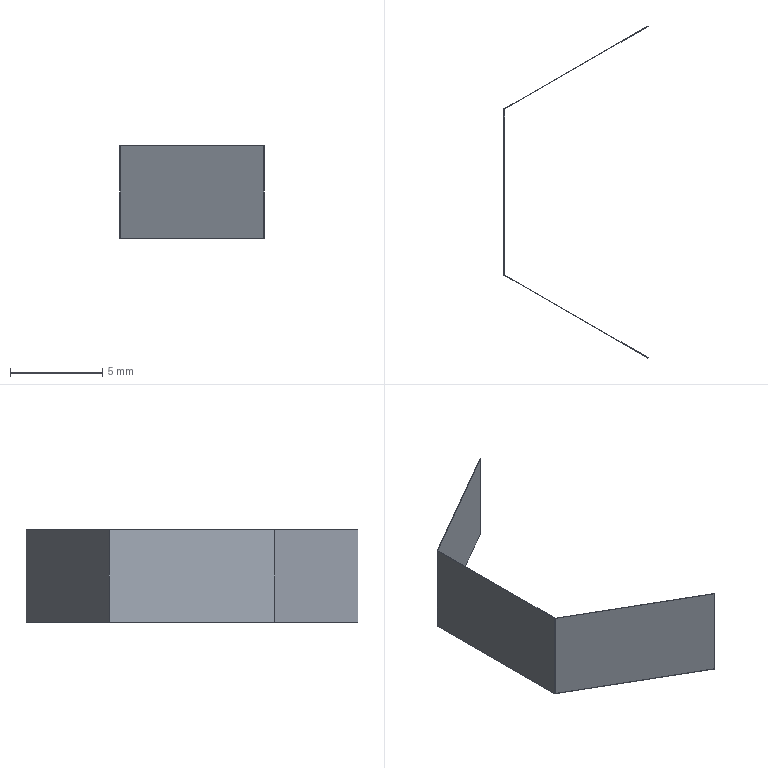Part | STEP file | 1 solid | 10 faces | box 7.817 x 18 x 5 mm | volume 4.038 mm3 | plane 10
STEP:
#1=CARTESIAN_POINT('',(0.,0.,0.));
#2=DIRECTION('',(0.,0.,1.));
#3=DIRECTION('',(1.,0.,0.));
#4=AXIS2_PLACEMENT_3D('',#1,#2,#3);
#5=CARTESIAN_POINT('',(23.783,162.32,44.99));
#6=VERTEX_POINT('',#5);
#7=CARTESIAN_POINT('',(23.783,162.32,39.99));
#8=VERTEX_POINT('',#7);
#9=CARTESIAN_POINT('',(23.783,162.32,44.99));
#10=DIRECTION('',(0.,0.,-1.));
#11=VECTOR('',#10,1.);
#12=LINE('',#9,#11);
#13=CARTESIAN_POINT('',(31.577,166.82,44.99));
#14=DIRECTION('',(0.5,-0.866,0.));
#15=DIRECTION('',(0.866,0.5,0.));
#16=AXIS2_PLACEMENT_3D('',#13,#14,#15);
#17=PLANE('',#16);
#18=CARTESIAN_POINT('',(-9.,0.));
#19=DIRECTION('',(0.,-1.));
#20=VECTOR('',#19,1.);
#21=LINE('',#18,#20);
#22=(GEOMETRIC_REPRESENTATION_CONTEXT(2)PARAMETRIC_REPRESENTATION_CONTEXT()REPRESENTATION_CONTEXT('',''));
#23=DEFINITIONAL_REPRESENTATION('',(#21),#22);
#24=PCURVE('',#17,#23);
#25=CARTESIAN_POINT('',(23.783,162.32,44.99));
#26=DIRECTION('',(1.,0.,0.));
#27=DIRECTION('',(0.,0.,-1.));
#28=AXIS2_PLACEMENT_3D('',#25,#26,#27);
#29=PLANE('',#28);
#30=CARTESIAN_POINT('',(0.,0.));
#31=DIRECTION('',(1.,0.));
#32=VECTOR('',#31,1.);
#33=LINE('',#30,#32);
#34=(GEOMETRIC_REPRESENTATION_CONTEXT(2)PARAMETRIC_REPRESENTATION_CONTEXT()REPRESENTATION_CONTEXT('',''));
#35=DEFINITIONAL_REPRESENTATION('',(#33),#34);
#36=PCURVE('',#29,#35);
#37=SURFACE_CURVE('',#12,(#24,#36),.PCURVE_S1.);
#38=EDGE_CURVE('',#6,#8,#37,.T.);
#39=ORIENTED_EDGE('',*,*,#38,.F.);
#40=CARTESIAN_POINT('',(31.577,166.82,44.99));
#41=VERTEX_POINT('',#40);
#42=CARTESIAN_POINT('',(31.577,166.82,44.99));
#43=DIRECTION('',(-0.866,-0.5,0.));
#44=VECTOR('',#43,1.);
#45=LINE('',#42,#44);
#46=CARTESIAN_POINT('',(0.,0.));
#47=DIRECTION('',(-1.,0.));
#48=VECTOR('',#47,1.);
#49=LINE('',#46,#48);
#50=(GEOMETRIC_REPRESENTATION_CONTEXT(2)PARAMETRIC_REPRESENTATION_CONTEXT()REPRESENTATION_CONTEXT('',''));
#51=DEFINITIONAL_REPRESENTATION('',(#49),#50);
#52=PCURVE('',#17,#51);
#53=CARTESIAN_POINT('',(31.622,157.82,44.99));
#54=DIRECTION('',(0.,0.,-1.));
#55=DIRECTION('',(-1.,0.,0.));
#56=AXIS2_PLACEMENT_3D('',#53,#54,#55);
#57=PLANE('',#56);
#58=CARTESIAN_POINT('',(0.0449,9.));
#59=DIRECTION('',(0.866,-0.5));
#60=VECTOR('',#59,1.);
#61=LINE('',#58,#60);
#62=(GEOMETRIC_REPRESENTATION_CONTEXT(2)PARAMETRIC_REPRESENTATION_CONTEXT()REPRESENTATION_CONTEXT('',''));
#63=DEFINITIONAL_REPRESENTATION('',(#61),#62);
#64=PCURVE('',#57,#63);
#65=SURFACE_CURVE('',#45,(#52,#64),.PCURVE_S1.);
#66=EDGE_CURVE('',#41,#6,#65,.T.);
#67=ORIENTED_EDGE('',*,*,#66,.F.);
#68=CARTESIAN_POINT('',(31.577,166.82,39.99));
#69=VERTEX_POINT('',#68);
#70=CARTESIAN_POINT('',(31.577,166.82,44.99));
#71=DIRECTION('',(0.,0.,1.));
#72=VECTOR('',#71,1.);
#73=LINE('',#70,#72);
#74=CARTESIAN_POINT('',(0.,0.));
#75=DIRECTION('',(0.,1.));
#76=VECTOR('',#75,1.);
#77=LINE('',#74,#76);
#78=(GEOMETRIC_REPRESENTATION_CONTEXT(2)PARAMETRIC_REPRESENTATION_CONTEXT()REPRESENTATION_CONTEXT('',''));
#79=DEFINITIONAL_REPRESENTATION('',(#77),#78);
#80=PCURVE('',#17,#79);
#81=CARTESIAN_POINT('',(39.371,162.32,44.99));
#82=DIRECTION('',(-0.5,-0.866,0.));
#83=DIRECTION('',(0.866,-0.5,0.));
#84=AXIS2_PLACEMENT_3D('',#81,#82,#83);
#85=PLANE('',#84);
#86=CARTESIAN_POINT('',(-9.,0.));
#87=DIRECTION('',(0.,1.));
#88=VECTOR('',#87,1.);
#89=LINE('',#86,#88);
#90=(GEOMETRIC_REPRESENTATION_CONTEXT(2)PARAMETRIC_REPRESENTATION_CONTEXT()REPRESENTATION_CONTEXT('',''));
#91=DEFINITIONAL_REPRESENTATION('',(#89),#90);
#92=PCURVE('',#85,#91);
#93=SURFACE_CURVE('',#73,(#80,#92),.PCURVE_S1.);
#94=EDGE_CURVE('',#69,#41,#93,.T.);
#95=ORIENTED_EDGE('',*,*,#94,.F.);
#96=CARTESIAN_POINT('',(31.577,166.82,39.99));
#97=DIRECTION('',(0.866,0.5,0.));
#98=VECTOR('',#97,1.);
#99=LINE('',#96,#98);
#100=CARTESIAN_POINT('',(0.,-5.));
#101=DIRECTION('',(1.,0.));
#102=VECTOR('',#101,1.);
#103=LINE('',#100,#102);
#104=(GEOMETRIC_REPRESENTATION_CONTEXT(2)PARAMETRIC_REPRESENTATION_CONTEXT()REPRESENTATION_CONTEXT('',''));
#105=DEFINITIONAL_REPRESENTATION('',(#103),#104);
#106=PCURVE('',#17,#105);
#107=CARTESIAN_POINT('',(31.622,166.745,39.99));
#108=DIRECTION('',(0.,0.,1.));
#109=DIRECTION('',(1.,0.,0.));
#110=AXIS2_PLACEMENT_3D('',#107,#108,#109);
#111=PLANE('',#110);
#112=CARTESIAN_POINT('',(-0.0449,0.075));
#113=DIRECTION('',(0.866,0.5));
#114=VECTOR('',#113,1.);
#115=LINE('',#112,#114);
#116=(GEOMETRIC_REPRESENTATION_CONTEXT(2)PARAMETRIC_REPRESENTATION_CONTEXT()REPRESENTATION_CONTEXT('',''));
#117=DEFINITIONAL_REPRESENTATION('',(#115),#116);
#118=PCURVE('',#111,#117);
#119=SURFACE_CURVE('',#99,(#106,#118),.PCURVE_S1.);
#120=EDGE_CURVE('',#8,#69,#119,.T.);
#121=ORIENTED_EDGE('',*,*,#120,.F.);
#122=EDGE_LOOP('',(#39,#67,#95,#121));
#123=FACE_BOUND('',#122,.T.);
#124=ADVANCED_FACE('',(#123),#17,.F.);
#125=CARTESIAN_POINT('',(23.783,153.32,39.99));
#126=VERTEX_POINT('',#125);
#127=CARTESIAN_POINT('',(31.577,148.82,39.99));
#128=VERTEX_POINT('',#127);
#129=CARTESIAN_POINT('',(23.783,153.32,39.99));
#130=DIRECTION('',(0.866,-0.5,0.));
#131=VECTOR('',#130,1.);
#132=LINE('',#129,#131);
#133=CARTESIAN_POINT('',(-7.839,-13.425));
#134=DIRECTION('',(0.866,-0.5));
#135=VECTOR('',#134,1.);
#136=LINE('',#133,#135);
#137=(GEOMETRIC_REPRESENTATION_CONTEXT(2)PARAMETRIC_REPRESENTATION_CONTEXT()REPRESENTATION_CONTEXT('',''));
#138=DEFINITIONAL_REPRESENTATION('',(#136),#137);
#139=PCURVE('',#111,#138);
#140=CARTESIAN_POINT('',(23.783,153.32,44.99));
#141=DIRECTION('',(0.5,0.866,0.));
#142=DIRECTION('',(-0.866,0.5,0.));
#143=AXIS2_PLACEMENT_3D('',#140,#141,#142);
#144=PLANE('',#143);
#145=CARTESIAN_POINT('',(0.,-5.));
#146=DIRECTION('',(-1.,0.));
#147=VECTOR('',#146,1.);
#148=LINE('',#145,#147);
#149=(GEOMETRIC_REPRESENTATION_CONTEXT(2)PARAMETRIC_REPRESENTATION_CONTEXT()REPRESENTATION_CONTEXT('',''));
#150=DEFINITIONAL_REPRESENTATION('',(#148),#149);
#151=PCURVE('',#144,#150);
#152=SURFACE_CURVE('',#132,(#139,#151),.PCURVE_S1.);
#153=EDGE_CURVE('',#126,#128,#152,.T.);
#154=ORIENTED_EDGE('',*,*,#153,.F.);
#155=CARTESIAN_POINT('',(23.783,166.745,39.99));
#156=DIRECTION('',(0.,-1.,0.));
#157=VECTOR('',#156,1.);
#158=LINE('',#155,#157);
#159=CARTESIAN_POINT('',(-7.839,0.));
#160=DIRECTION('',(0.,-1.));
#161=VECTOR('',#160,1.);
#162=LINE('',#159,#161);
#163=(GEOMETRIC_REPRESENTATION_CONTEXT(2)PARAMETRIC_REPRESENTATION_CONTEXT()REPRESENTATION_CONTEXT('',''));
#164=DEFINITIONAL_REPRESENTATION('',(#162),#163);
#165=PCURVE('',#111,#164);
#166=CARTESIAN_POINT('',(5.,4.425));
#167=DIRECTION('',(0.,-1.));
#168=VECTOR('',#167,1.);
#169=LINE('',#166,#168);
#170=(GEOMETRIC_REPRESENTATION_CONTEXT(2)PARAMETRIC_REPRESENTATION_CONTEXT()REPRESENTATION_CONTEXT('',''));
#171=DEFINITIONAL_REPRESENTATION('',(#169),#170);
#172=PCURVE('',#29,#171);
#173=SURFACE_CURVE('',#158,(#165,#172),.PCURVE_S1.);
#174=EDGE_CURVE('',#8,#126,#173,.T.);
#175=ORIENTED_EDGE('',*,*,#174,.F.);
#176=ORIENTED_EDGE('',*,*,#120,.T.);
#177=CARTESIAN_POINT('',(31.6,166.807,39.99));
#178=VERTEX_POINT('',#177);
#179=CARTESIAN_POINT('',(31.6,166.807,39.99));
#180=DIRECTION('',(-0.866,0.5,0.));
#181=VECTOR('',#180,1.);
#182=LINE('',#179,#181);
#183=CARTESIAN_POINT('',(-0.02245,0.06204));
#184=DIRECTION('',(-0.866,0.5));
#185=VECTOR('',#184,1.);
#186=LINE('',#183,#185);
#187=(GEOMETRIC_REPRESENTATION_CONTEXT(2)PARAMETRIC_REPRESENTATION_CONTEXT()REPRESENTATION_CONTEXT('',''));
#188=DEFINITIONAL_REPRESENTATION('',(#186),#187);
#189=PCURVE('',#111,#188);
#190=CARTESIAN_POINT('',(-8.974,-5.));
#191=DIRECTION('',(-1.,0.));
#192=VECTOR('',#191,1.);
#193=LINE('',#190,#192);
#194=(GEOMETRIC_REPRESENTATION_CONTEXT(2)PARAMETRIC_REPRESENTATION_CONTEXT()REPRESENTATION_CONTEXT('',''));
#195=DEFINITIONAL_REPRESENTATION('',(#193),#194);
#196=PCURVE('',#85,#195);
#197=SURFACE_CURVE('',#182,(#189,#196),.PCURVE_S1.);
#198=EDGE_CURVE('',#178,#69,#197,.T.);
#199=ORIENTED_EDGE('',*,*,#198,.F.);
#200=CARTESIAN_POINT('',(23.828,162.32,39.99));
#201=VERTEX_POINT('',#200);
#202=CARTESIAN_POINT('',(23.828,162.32,39.99));
#203=DIRECTION('',(0.866,0.5,0.));
#204=VECTOR('',#203,1.);
#205=LINE('',#202,#204);
#206=CARTESIAN_POINT('',(-7.794,-4.425));
#207=DIRECTION('',(0.866,0.5));
#208=VECTOR('',#207,1.);
#209=LINE('',#206,#208);
#210=(GEOMETRIC_REPRESENTATION_CONTEXT(2)PARAMETRIC_REPRESENTATION_CONTEXT()REPRESENTATION_CONTEXT('',''));
#211=DEFINITIONAL_REPRESENTATION('',(#209),#210);
#212=PCURVE('',#111,#211);
#213=CARTESIAN_POINT('',(23.828,162.32,39.99));
#214=DIRECTION('',(-0.5,0.866,0.));
#215=DIRECTION('',(-0.866,-0.5,0.));
#216=AXIS2_PLACEMENT_3D('',#213,#214,#215);
#217=PLANE('',#216);
#218=CARTESIAN_POINT('',(0.,0.));
#219=DIRECTION('',(-1.,0.));
#220=VECTOR('',#219,1.);
#221=LINE('',#218,#220);
#222=(GEOMETRIC_REPRESENTATION_CONTEXT(2)PARAMETRIC_REPRESENTATION_CONTEXT()REPRESENTATION_CONTEXT('',''));
#223=DEFINITIONAL_REPRESENTATION('',(#221),#222);
#224=PCURVE('',#217,#223);
#225=SURFACE_CURVE('',#205,(#212,#224),.PCURVE_S1.);
#226=EDGE_CURVE('',#201,#178,#225,.T.);
#227=ORIENTED_EDGE('',*,*,#226,.F.);
#228=CARTESIAN_POINT('',(23.828,153.32,39.99));
#229=VERTEX_POINT('',#228);
#230=CARTESIAN_POINT('',(23.828,166.745,39.99));
#231=DIRECTION('',(0.,1.,0.));
#232=VECTOR('',#231,1.);
#233=LINE('',#230,#232);
#234=CARTESIAN_POINT('',(-7.794,0.));
#235=DIRECTION('',(0.,1.));
#236=VECTOR('',#235,1.);
#237=LINE('',#234,#236);
#238=(GEOMETRIC_REPRESENTATION_CONTEXT(2)PARAMETRIC_REPRESENTATION_CONTEXT()REPRESENTATION_CONTEXT('',''));
#239=DEFINITIONAL_REPRESENTATION('',(#237),#238);
#240=PCURVE('',#111,#239);
#241=CARTESIAN_POINT('',(23.828,153.32,39.99));
#242=DIRECTION('',(-1.,0.,0.));
#243=DIRECTION('',(0.,0.,1.));
#244=AXIS2_PLACEMENT_3D('',#241,#242,#243);
#245=PLANE('',#244);
#246=CARTESIAN_POINT('',(0.,13.425));
#247=DIRECTION('',(0.,1.));
#248=VECTOR('',#247,1.);
#249=LINE('',#246,#248);
#250=(GEOMETRIC_REPRESENTATION_CONTEXT(2)PARAMETRIC_REPRESENTATION_CONTEXT()REPRESENTATION_CONTEXT('',''));
#251=DEFINITIONAL_REPRESENTATION('',(#249),#250);
#252=PCURVE('',#245,#251);
#253=SURFACE_CURVE('',#233,(#240,#252),.PCURVE_S1.);
#254=EDGE_CURVE('',#229,#201,#253,.T.);
#255=ORIENTED_EDGE('',*,*,#254,.F.);
#256=CARTESIAN_POINT('',(31.6,148.833,39.99));
#257=VERTEX_POINT('',#256);
#258=CARTESIAN_POINT('',(31.6,148.833,39.99));
#259=DIRECTION('',(-0.866,0.5,0.));
#260=VECTOR('',#259,1.);
#261=LINE('',#258,#260);
#262=CARTESIAN_POINT('',(-0.02245,-17.912));
#263=DIRECTION('',(-0.866,0.5));
#264=VECTOR('',#263,1.);
#265=LINE('',#262,#264);
#266=(GEOMETRIC_REPRESENTATION_CONTEXT(2)PARAMETRIC_REPRESENTATION_CONTEXT()REPRESENTATION_CONTEXT('',''));
#267=DEFINITIONAL_REPRESENTATION('',(#265),#266);
#268=PCURVE('',#111,#267);
#269=CARTESIAN_POINT('',(31.622,148.82,39.99));
#270=DIRECTION('',(-0.5,-0.866,0.));
#271=DIRECTION('',(0.866,-0.5,0.));
#272=AXIS2_PLACEMENT_3D('',#269,#270,#271);
#273=PLANE('',#272);
#274=CARTESIAN_POINT('',(-0.02592,0.));
#275=DIRECTION('',(-1.,0.));
#276=VECTOR('',#275,1.);
#277=LINE('',#274,#276);
#278=(GEOMETRIC_REPRESENTATION_CONTEXT(2)PARAMETRIC_REPRESENTATION_CONTEXT()REPRESENTATION_CONTEXT('',''));
#279=DEFINITIONAL_REPRESENTATION('',(#277),#278);
#280=PCURVE('',#273,#279);
#281=SURFACE_CURVE('',#261,(#268,#280),.PCURVE_S1.);
#282=EDGE_CURVE('',#257,#229,#281,.T.);
#283=ORIENTED_EDGE('',*,*,#282,.F.);
#284=CARTESIAN_POINT('',(31.577,148.82,39.99));
#285=DIRECTION('',(-0.866,-0.5,0.));
#286=VECTOR('',#285,1.);
#287=LINE('',#284,#286);
#288=CARTESIAN_POINT('',(-0.0449,-17.925));
#289=DIRECTION('',(-0.866,-0.5));
#290=VECTOR('',#289,1.);
#291=LINE('',#288,#290);
#292=(GEOMETRIC_REPRESENTATION_CONTEXT(2)PARAMETRIC_REPRESENTATION_CONTEXT()REPRESENTATION_CONTEXT('',''));
#293=DEFINITIONAL_REPRESENTATION('',(#291),#292);
#294=PCURVE('',#111,#293);
#295=CARTESIAN_POINT('',(31.577,148.82,44.99));
#296=DIRECTION('',(-0.5,0.866,0.));
#297=DIRECTION('',(-0.866,-0.5,0.));
#298=AXIS2_PLACEMENT_3D('',#295,#296,#297);
#299=PLANE('',#298);
#300=CARTESIAN_POINT('',(0.,-5.));
#301=DIRECTION('',(1.,0.));
#302=VECTOR('',#301,1.);
#303=LINE('',#300,#302);
#304=(GEOMETRIC_REPRESENTATION_CONTEXT(2)PARAMETRIC_REPRESENTATION_CONTEXT()REPRESENTATION_CONTEXT('',''));
#305=DEFINITIONAL_REPRESENTATION('',(#303),#304);
#306=PCURVE('',#299,#305);
#307=SURFACE_CURVE('',#287,(#294,#306),.PCURVE_S1.);
#308=EDGE_CURVE('',#257,#128,#307,.T.);
#309=ORIENTED_EDGE('',*,*,#308,.T.);
#310=EDGE_LOOP('',(#154,#175,#176,#199,#227,#255,#283,#309));
#311=FACE_BOUND('',#310,.T.);
#312=ADVANCED_FACE('',(#311),#111,.F.);
#313=CARTESIAN_POINT('',(23.783,153.32,44.99));
#314=VERTEX_POINT('',#313);
#315=CARTESIAN_POINT('',(23.783,153.32,44.99));
#316=DIRECTION('',(0.,0.,-1.));
#317=VECTOR('',#316,1.);
#318=LINE('',#315,#317);
#319=CARTESIAN_POINT('',(0.,-9.));
#320=DIRECTION('',(1.,0.));
#321=VECTOR('',#320,1.);
#322=LINE('',#319,#321);
#323=(GEOMETRIC_REPRESENTATION_CONTEXT(2)PARAMETRIC_REPRESENTATION_CONTEXT()REPRESENTATION_CONTEXT('',''));
#324=DEFINITIONAL_REPRESENTATION('',(#322),#323);
#325=PCURVE('',#29,#324);
#326=CARTESIAN_POINT('',(0.,0.));
#327=DIRECTION('',(0.,-1.));
#328=VECTOR('',#327,1.);
#329=LINE('',#326,#328);
#330=(GEOMETRIC_REPRESENTATION_CONTEXT(2)PARAMETRIC_REPRESENTATION_CONTEXT()REPRESENTATION_CONTEXT('',''));
#331=DEFINITIONAL_REPRESENTATION('',(#329),#330);
#332=PCURVE('',#144,#331);
#333=SURFACE_CURVE('',#318,(#325,#332),.PCURVE_S1.);
#334=EDGE_CURVE('',#314,#126,#333,.T.);
#335=ORIENTED_EDGE('',*,*,#334,.F.);
#336=CARTESIAN_POINT('',(23.783,162.32,44.99));
#337=DIRECTION('',(0.,-1.,0.));
#338=VECTOR('',#337,1.);
#339=LINE('',#336,#338);
#340=CARTESIAN_POINT('',(0.,0.));
#341=DIRECTION('',(0.,-1.));
#342=VECTOR('',#341,1.);
#343=LINE('',#340,#342);
#344=(GEOMETRIC_REPRESENTATION_CONTEXT(2)PARAMETRIC_REPRESENTATION_CONTEXT()REPRESENTATION_CONTEXT('',''));
#345=DEFINITIONAL_REPRESENTATION('',(#343),#344);
#346=PCURVE('',#29,#345);
#347=CARTESIAN_POINT('',(7.839,4.5));
#348=DIRECTION('',(0.,-1.));
#349=VECTOR('',#348,1.);
#350=LINE('',#347,#349);
#351=(GEOMETRIC_REPRESENTATION_CONTEXT(2)PARAMETRIC_REPRESENTATION_CONTEXT()REPRESENTATION_CONTEXT('',''));
#352=DEFINITIONAL_REPRESENTATION('',(#350),#351);
#353=PCURVE('',#57,#352);
#354=SURFACE_CURVE('',#339,(#346,#353),.PCURVE_S1.);
#355=EDGE_CURVE('',#6,#314,#354,.T.);
#356=ORIENTED_EDGE('',*,*,#355,.F.);
#357=ORIENTED_EDGE('',*,*,#38,.T.);
#358=ORIENTED_EDGE('',*,*,#174,.T.);
#359=EDGE_LOOP('',(#335,#356,#357,#358));
#360=FACE_BOUND('',#359,.T.);
#361=ADVANCED_FACE('',(#360),#29,.F.);
#362=CARTESIAN_POINT('',(23.828,153.32,44.99));
#363=VERTEX_POINT('',#362);
#364=CARTESIAN_POINT('',(31.6,148.833,44.99));
#365=VERTEX_POINT('',#364);
#366=CARTESIAN_POINT('',(23.828,153.32,44.99));
#367=DIRECTION('',(0.866,-0.5,0.));
#368=VECTOR('',#367,1.);
#369=LINE('',#366,#368);
#370=CARTESIAN_POINT('',(7.794,-4.5));
#371=DIRECTION('',(-0.866,-0.5));
#372=VECTOR('',#371,1.);
#373=LINE('',#370,#372);
#374=(GEOMETRIC_REPRESENTATION_CONTEXT(2)PARAMETRIC_REPRESENTATION_CONTEXT()REPRESENTATION_CONTEXT('',''));
#375=DEFINITIONAL_REPRESENTATION('',(#373),#374);
#376=PCURVE('',#57,#375);
#377=CARTESIAN_POINT('',(-9.,5.));
#378=DIRECTION('',(1.,0.));
#379=VECTOR('',#378,1.);
#380=LINE('',#377,#379);
#381=(GEOMETRIC_REPRESENTATION_CONTEXT(2)PARAMETRIC_REPRESENTATION_CONTEXT()REPRESENTATION_CONTEXT('',''));
#382=DEFINITIONAL_REPRESENTATION('',(#380),#381);
#383=PCURVE('',#273,#382);
#384=SURFACE_CURVE('',#369,(#376,#383),.PCURVE_S1.);
#385=EDGE_CURVE('',#363,#365,#384,.T.);
#386=ORIENTED_EDGE('',*,*,#385,.F.);
#387=CARTESIAN_POINT('',(23.828,162.32,44.99));
#388=VERTEX_POINT('',#387);
#389=CARTESIAN_POINT('',(23.828,157.82,44.99));
#390=DIRECTION('',(0.,-1.,0.));
#391=VECTOR('',#390,1.);
#392=LINE('',#389,#391);
#393=CARTESIAN_POINT('',(7.794,0.));
#394=DIRECTION('',(0.,-1.));
#395=VECTOR('',#394,1.);
#396=LINE('',#393,#395);
#397=(GEOMETRIC_REPRESENTATION_CONTEXT(2)PARAMETRIC_REPRESENTATION_CONTEXT()REPRESENTATION_CONTEXT('',''));
#398=DEFINITIONAL_REPRESENTATION('',(#396),#397);
#399=PCURVE('',#57,#398);
#400=CARTESIAN_POINT('',(5.,4.5));
#401=DIRECTION('',(0.,-1.));
#402=VECTOR('',#401,1.);
#403=LINE('',#400,#402);
#404=(GEOMETRIC_REPRESENTATION_CONTEXT(2)PARAMETRIC_REPRESENTATION_CONTEXT()REPRESENTATION_CONTEXT('',''));
#405=DEFINITIONAL_REPRESENTATION('',(#403),#404);
#406=PCURVE('',#245,#405);
#407=SURFACE_CURVE('',#392,(#399,#406),.PCURVE_S1.);
#408=EDGE_CURVE('',#388,#363,#407,.T.);
#409=ORIENTED_EDGE('',*,*,#408,.F.);
#410=CARTESIAN_POINT('',(31.6,166.807,44.99));
#411=VERTEX_POINT('',#410);
#412=CARTESIAN_POINT('',(31.6,166.807,44.99));
#413=DIRECTION('',(-0.866,-0.5,0.));
#414=VECTOR('',#413,1.);
#415=LINE('',#412,#414);
#416=CARTESIAN_POINT('',(0.02245,8.987));
#417=DIRECTION('',(0.866,-0.5));
#418=VECTOR('',#417,1.);
#419=LINE('',#416,#418);
#420=(GEOMETRIC_REPRESENTATION_CONTEXT(2)PARAMETRIC_REPRESENTATION_CONTEXT()REPRESENTATION_CONTEXT('',''));
#421=DEFINITIONAL_REPRESENTATION('',(#419),#420);
#422=PCURVE('',#57,#421);
#423=CARTESIAN_POINT('',(-8.974,5.));
#424=DIRECTION('',(1.,0.));
#425=VECTOR('',#424,1.);
#426=LINE('',#423,#425);
#427=(GEOMETRIC_REPRESENTATION_CONTEXT(2)PARAMETRIC_REPRESENTATION_CONTEXT()REPRESENTATION_CONTEXT('',''));
#428=DEFINITIONAL_REPRESENTATION('',(#426),#427);
#429=PCURVE('',#217,#428);
#430=SURFACE_CURVE('',#415,(#422,#429),.PCURVE_S1.);
#431=EDGE_CURVE('',#411,#388,#430,.T.);
#432=ORIENTED_EDGE('',*,*,#431,.F.);
#433=CARTESIAN_POINT('',(31.577,166.82,44.99));
#434=DIRECTION('',(0.866,-0.5,0.));
#435=VECTOR('',#434,1.);
#436=LINE('',#433,#435);
#437=CARTESIAN_POINT('',(0.0449,9.));
#438=DIRECTION('',(-0.866,-0.5));
#439=VECTOR('',#438,1.);
#440=LINE('',#437,#439);
#441=(GEOMETRIC_REPRESENTATION_CONTEXT(2)PARAMETRIC_REPRESENTATION_CONTEXT()REPRESENTATION_CONTEXT('',''));
#442=DEFINITIONAL_REPRESENTATION('',(#440),#441);
#443=PCURVE('',#57,#442);
#444=CARTESIAN_POINT('',(-9.,0.));
#445=DIRECTION('',(1.,0.));
#446=VECTOR('',#445,1.);
#447=LINE('',#444,#446);
#448=(GEOMETRIC_REPRESENTATION_CONTEXT(2)PARAMETRIC_REPRESENTATION_CONTEXT()REPRESENTATION_CONTEXT('',''));
#449=DEFINITIONAL_REPRESENTATION('',(#447),#448);
#450=PCURVE('',#85,#449);
#451=SURFACE_CURVE('',#436,(#443,#450),.PCURVE_S1.);
#452=EDGE_CURVE('',#41,#411,#451,.T.);
#453=ORIENTED_EDGE('',*,*,#452,.F.);
#454=ORIENTED_EDGE('',*,*,#66,.T.);
#455=ORIENTED_EDGE('',*,*,#355,.T.);
#456=CARTESIAN_POINT('',(31.577,148.82,44.99));
#457=VERTEX_POINT('',#456);
#458=CARTESIAN_POINT('',(31.577,148.82,44.99));
#459=DIRECTION('',(-0.866,0.5,0.));
#460=VECTOR('',#459,1.);
#461=LINE('',#458,#460);
#462=CARTESIAN_POINT('',(0.0449,-9.));
#463=DIRECTION('',(0.866,0.5));
#464=VECTOR('',#463,1.);
#465=LINE('',#462,#464);
#466=(GEOMETRIC_REPRESENTATION_CONTEXT(2)PARAMETRIC_REPRESENTATION_CONTEXT()REPRESENTATION_CONTEXT('',''));
#467=DEFINITIONAL_REPRESENTATION('',(#465),#466);
#468=PCURVE('',#57,#467);
#469=CARTESIAN_POINT('',(-9.,0.));
#470=DIRECTION('',(1.,0.));
#471=VECTOR('',#470,1.);
#472=LINE('',#469,#471);
#473=(GEOMETRIC_REPRESENTATION_CONTEXT(2)PARAMETRIC_REPRESENTATION_CONTEXT()REPRESENTATION_CONTEXT('',''));
#474=DEFINITIONAL_REPRESENTATION('',(#472),#473);
#475=PCURVE('',#144,#474);
#476=SURFACE_CURVE('',#461,(#468,#475),.PCURVE_S1.);
#477=EDGE_CURVE('',#457,#314,#476,.T.);
#478=ORIENTED_EDGE('',*,*,#477,.F.);
#479=CARTESIAN_POINT('',(31.577,148.82,44.99));
#480=DIRECTION('',(0.866,0.5,0.));
#481=VECTOR('',#480,1.);
#482=LINE('',#479,#481);
#483=CARTESIAN_POINT('',(0.0449,-9.));
#484=DIRECTION('',(-0.866,0.5));
#485=VECTOR('',#484,1.);
#486=LINE('',#483,#485);
#487=(GEOMETRIC_REPRESENTATION_CONTEXT(2)PARAMETRIC_REPRESENTATION_CONTEXT()REPRESENTATION_CONTEXT('',''));
#488=DEFINITIONAL_REPRESENTATION('',(#486),#487);
#489=PCURVE('',#57,#488);
#490=CARTESIAN_POINT('',(0.,0.));
#491=DIRECTION('',(-1.,0.));
#492=VECTOR('',#491,1.);
#493=LINE('',#490,#492);
#494=(GEOMETRIC_REPRESENTATION_CONTEXT(2)PARAMETRIC_REPRESENTATION_CONTEXT()REPRESENTATION_CONTEXT('',''));
#495=DEFINITIONAL_REPRESENTATION('',(#493),#494);
#496=PCURVE('',#299,#495);
#497=SURFACE_CURVE('',#482,(#489,#496),.PCURVE_S1.);
#498=EDGE_CURVE('',#457,#365,#497,.T.);
#499=ORIENTED_EDGE('',*,*,#498,.T.);
#500=EDGE_LOOP('',(#386,#409,#432,#453,#454,#455,#478,#499));
#501=FACE_BOUND('',#500,.T.);
#502=ADVANCED_FACE('',(#501),#57,.F.);
#503=ORIENTED_EDGE('',*,*,#198,.T.);
#504=ORIENTED_EDGE('',*,*,#94,.T.);
#505=ORIENTED_EDGE('',*,*,#452,.T.);
#506=CARTESIAN_POINT('',(31.6,166.807,44.99));
#507=DIRECTION('',(0.,0.,1.));
#508=VECTOR('',#507,1.);
#509=LINE('',#506,#508);
#510=CARTESIAN_POINT('',(-8.974,0.));
#511=DIRECTION('',(0.,1.));
#512=VECTOR('',#511,1.);
#513=LINE('',#510,#512);
#514=(GEOMETRIC_REPRESENTATION_CONTEXT(2)PARAMETRIC_REPRESENTATION_CONTEXT()REPRESENTATION_CONTEXT('',''));
#515=DEFINITIONAL_REPRESENTATION('',(#513),#514);
#516=PCURVE('',#85,#515);
#517=CARTESIAN_POINT('',(-8.974,5.));
#518=DIRECTION('',(0.,1.));
#519=VECTOR('',#518,1.);
#520=LINE('',#517,#519);
#521=(GEOMETRIC_REPRESENTATION_CONTEXT(2)PARAMETRIC_REPRESENTATION_CONTEXT()REPRESENTATION_CONTEXT('',''));
#522=DEFINITIONAL_REPRESENTATION('',(#520),#521);
#523=PCURVE('',#217,#522);
#524=SURFACE_CURVE('',#509,(#516,#523),.PCURVE_S1.);
#525=EDGE_CURVE('',#178,#411,#524,.T.);
#526=ORIENTED_EDGE('',*,*,#525,.F.);
#527=EDGE_LOOP('',(#503,#504,#505,#526));
#528=FACE_BOUND('',#527,.T.);
#529=ADVANCED_FACE('',(#528),#85,.F.);
#530=CARTESIAN_POINT('',(31.577,148.82,44.99));
#531=DIRECTION('',(0.,0.,-1.));
#532=VECTOR('',#531,1.);
#533=LINE('',#530,#532);
#534=CARTESIAN_POINT('',(-9.,0.));
#535=DIRECTION('',(0.,-1.));
#536=VECTOR('',#535,1.);
#537=LINE('',#534,#536);
#538=(GEOMETRIC_REPRESENTATION_CONTEXT(2)PARAMETRIC_REPRESENTATION_CONTEXT()REPRESENTATION_CONTEXT('',''));
#539=DEFINITIONAL_REPRESENTATION('',(#537),#538);
#540=PCURVE('',#144,#539);
#541=CARTESIAN_POINT('',(0.,0.));
#542=DIRECTION('',(0.,-1.));
#543=VECTOR('',#542,1.);
#544=LINE('',#541,#543);
#545=(GEOMETRIC_REPRESENTATION_CONTEXT(2)PARAMETRIC_REPRESENTATION_CONTEXT()REPRESENTATION_CONTEXT('',''));
#546=DEFINITIONAL_REPRESENTATION('',(#544),#545);
#547=PCURVE('',#299,#546);
#548=SURFACE_CURVE('',#533,(#540,#547),.PCURVE_S1.);
#549=EDGE_CURVE('',#457,#128,#548,.T.);
#550=ORIENTED_EDGE('',*,*,#549,.F.);
#551=ORIENTED_EDGE('',*,*,#477,.T.);
#552=ORIENTED_EDGE('',*,*,#334,.T.);
#553=ORIENTED_EDGE('',*,*,#153,.T.);
#554=EDGE_LOOP('',(#550,#551,#552,#553));
#555=FACE_BOUND('',#554,.T.);
#556=ADVANCED_FACE('',(#555),#144,.F.);
#557=ORIENTED_EDGE('',*,*,#431,.T.);
#558=CARTESIAN_POINT('',(23.828,162.32,39.99));
#559=DIRECTION('',(0.,0.,1.));
#560=VECTOR('',#559,1.);
#561=LINE('',#558,#560);
#562=CARTESIAN_POINT('',(0.,0.));
#563=DIRECTION('',(0.,1.));
#564=VECTOR('',#563,1.);
#565=LINE('',#562,#564);
#566=(GEOMETRIC_REPRESENTATION_CONTEXT(2)PARAMETRIC_REPRESENTATION_CONTEXT()REPRESENTATION_CONTEXT('',''));
#567=DEFINITIONAL_REPRESENTATION('',(#565),#566);
#568=PCURVE('',#217,#567);
#569=CARTESIAN_POINT('',(0.,9.));
#570=DIRECTION('',(1.,0.));
#571=VECTOR('',#570,1.);
#572=LINE('',#569,#571);
#573=(GEOMETRIC_REPRESENTATION_CONTEXT(2)PARAMETRIC_REPRESENTATION_CONTEXT()REPRESENTATION_CONTEXT('',''));
#574=DEFINITIONAL_REPRESENTATION('',(#572),#573);
#575=PCURVE('',#245,#574);
#576=SURFACE_CURVE('',#561,(#568,#575),.PCURVE_S1.);
#577=EDGE_CURVE('',#201,#388,#576,.T.);
#578=ORIENTED_EDGE('',*,*,#577,.F.);
#579=ORIENTED_EDGE('',*,*,#226,.T.);
#580=ORIENTED_EDGE('',*,*,#525,.T.);
#581=EDGE_LOOP('',(#557,#578,#579,#580));
#582=FACE_BOUND('',#581,.T.);
#583=ADVANCED_FACE('',(#582),#217,.F.);
#584=CARTESIAN_POINT('',(23.828,153.32,39.99));
#585=DIRECTION('',(0.,0.,1.));
#586=VECTOR('',#585,1.);
#587=LINE('',#584,#586);
#588=CARTESIAN_POINT('',(0.,0.));
#589=DIRECTION('',(1.,0.));
#590=VECTOR('',#589,1.);
#591=LINE('',#588,#590);
#592=(GEOMETRIC_REPRESENTATION_CONTEXT(2)PARAMETRIC_REPRESENTATION_CONTEXT()REPRESENTATION_CONTEXT('',''));
#593=DEFINITIONAL_REPRESENTATION('',(#591),#592);
#594=PCURVE('',#245,#593);
#595=CARTESIAN_POINT('',(-9.,0.));
#596=DIRECTION('',(0.,1.));
#597=VECTOR('',#596,1.);
#598=LINE('',#595,#597);
#599=(GEOMETRIC_REPRESENTATION_CONTEXT(2)PARAMETRIC_REPRESENTATION_CONTEXT()REPRESENTATION_CONTEXT('',''));
#600=DEFINITIONAL_REPRESENTATION('',(#598),#599);
#601=PCURVE('',#273,#600);
#602=SURFACE_CURVE('',#587,(#594,#601),.PCURVE_S1.);
#603=EDGE_CURVE('',#229,#363,#602,.T.);
#604=ORIENTED_EDGE('',*,*,#603,.F.);
#605=ORIENTED_EDGE('',*,*,#254,.T.);
#606=ORIENTED_EDGE('',*,*,#577,.T.);
#607=ORIENTED_EDGE('',*,*,#408,.T.);
#608=EDGE_LOOP('',(#604,#605,#606,#607));
#609=FACE_BOUND('',#608,.T.);
#610=ADVANCED_FACE('',(#609),#245,.F.);
#611=ORIENTED_EDGE('',*,*,#282,.T.);
#612=ORIENTED_EDGE('',*,*,#603,.T.);
#613=ORIENTED_EDGE('',*,*,#385,.T.);
#614=CARTESIAN_POINT('',(31.6,148.833,39.99));
#615=DIRECTION('',(0.,0.,1.));
#616=VECTOR('',#615,1.);
#617=LINE('',#614,#616);
#618=CARTESIAN_POINT('',(-0.02592,0.));
#619=DIRECTION('',(0.,1.));
#620=VECTOR('',#619,1.);
#621=LINE('',#618,#620);
#622=(GEOMETRIC_REPRESENTATION_CONTEXT(2)PARAMETRIC_REPRESENTATION_CONTEXT()REPRESENTATION_CONTEXT('',''));
#623=DEFINITIONAL_REPRESENTATION('',(#621),#622);
#624=PCURVE('',#273,#623);
#625=CARTESIAN_POINT('',(-0.02592,-5.));
#626=DIRECTION('',(0.,1.));
#627=VECTOR('',#626,1.);
#628=LINE('',#625,#627);
#629=(GEOMETRIC_REPRESENTATION_CONTEXT(2)PARAMETRIC_REPRESENTATION_CONTEXT()REPRESENTATION_CONTEXT('',''));
#630=DEFINITIONAL_REPRESENTATION('',(#628),#629);
#631=PCURVE('',#299,#630);
#632=SURFACE_CURVE('',#617,(#624,#631),.PCURVE_S1.);
#633=EDGE_CURVE('',#257,#365,#632,.T.);
#634=ORIENTED_EDGE('',*,*,#633,.F.);
#635=EDGE_LOOP('',(#611,#612,#613,#634));
#636=FACE_BOUND('',#635,.T.);
#637=ADVANCED_FACE('',(#636),#273,.F.);
#638=ORIENTED_EDGE('',*,*,#498,.F.);
#639=ORIENTED_EDGE('',*,*,#549,.T.);
#640=ORIENTED_EDGE('',*,*,#308,.F.);
#641=ORIENTED_EDGE('',*,*,#633,.T.);
#642=EDGE_LOOP('',(#638,#639,#640,#641));
#643=FACE_BOUND('',#642,.T.);
#644=ADVANCED_FACE('',(#643),#299,.F.);
#645=CLOSED_SHELL('',(#124,#312,#361,#502,#529,#556,#583,#610,#637,#644));
#646=MANIFOLD_SOLID_BREP('',#645);
#647=(LENGTH_UNIT()NAMED_UNIT(*)SI_UNIT(.MILLI.,.METRE.));
#648=UNCERTAINTY_MEASURE_WITH_UNIT(LENGTH_MEASURE(0.0000001),#647,'','');
#649=(NAMED_UNIT(*)PLANE_ANGLE_UNIT()SI_UNIT($,.RADIAN.));
#650=(NAMED_UNIT(*)SI_UNIT($,.STERADIAN.)SOLID_ANGLE_UNIT());
#651=(GEOMETRIC_REPRESENTATION_CONTEXT(3)GLOBAL_UNCERTAINTY_ASSIGNED_CONTEXT((#648))GLOBAL_UNIT_ASSIGNED_CONTEXT((#647,#649,#650))REPRESENTATION_CONTEXT('',''));
#652=ADVANCED_BREP_SHAPE_REPRESENTATION('',(#4,#646),#651);